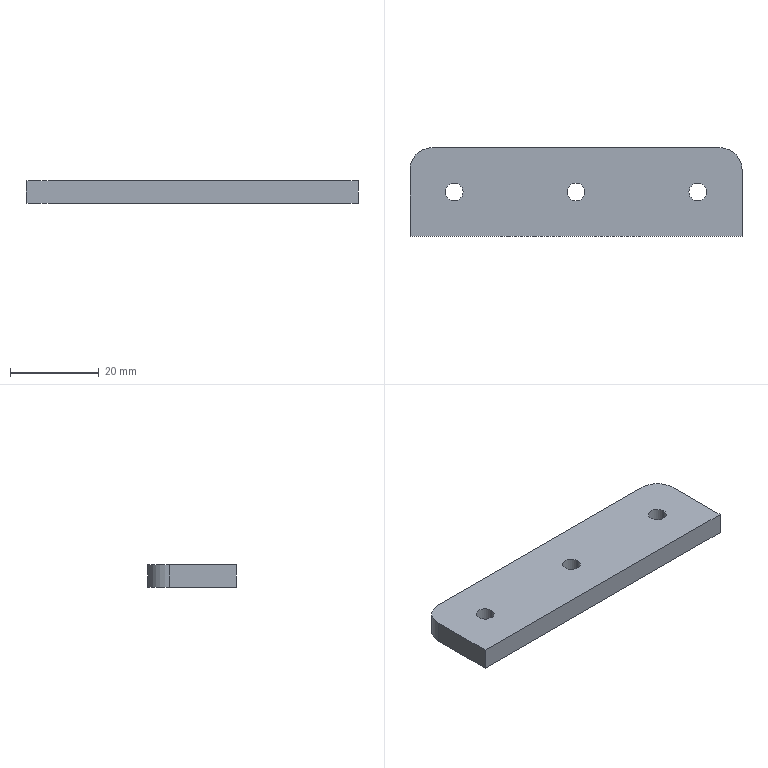Part | SolidWorks | features Extrusion 1, Fillet 1 | 1 solid | 14 faces | box 75 x 20 x 5 mm | volume 7258 mm3 | cylinder 8 | plane 6 | commonest cylinder face diameters 4 x6 10 x2
STEP:
#1=CARTESIAN_POINT('',(63.,-10.,5.));
#2=VERTEX_POINT('',#1);
#3=CARTESIAN_POINT('',(67.,-10.,5.));
#4=VERTEX_POINT('',#3);
#5=CARTESIAN_POINT('',(65.,-10.,5.));
#6=DIRECTION('',(0.,0.,1.));
#7=DIRECTION('',(1.,0.,0.));
#8=AXIS2_PLACEMENT_3D('',#5,#6,#7);
#9=CIRCLE('',#8,2.);
#10=EDGE_CURVE('',#2,#4,#9,.T.);
#11=ORIENTED_EDGE('',*,*,#10,.T.);
#12=CARTESIAN_POINT('',(67.,-10.,0.));
#13=VERTEX_POINT('',#12);
#14=CARTESIAN_POINT('',(67.,-10.,5.));
#15=DIRECTION('',(0.,0.,-1.));
#16=VECTOR('',#15,1000.);
#17=LINE('',#14,#16);
#18=EDGE_CURVE('',#4,#13,#17,.T.);
#19=ORIENTED_EDGE('',*,*,#18,.T.);
#20=CARTESIAN_POINT('',(63.,-10.,0.));
#21=VERTEX_POINT('',#20);
#22=CARTESIAN_POINT('',(65.,-10.,0.));
#23=DIRECTION('',(0.,0.,1.));
#24=DIRECTION('',(1.,0.,0.));
#25=AXIS2_PLACEMENT_3D('',#22,#23,#24);
#26=CIRCLE('',#25,2.);
#27=EDGE_CURVE('',#21,#13,#26,.T.);
#28=ORIENTED_EDGE('',*,*,#27,.F.);
#29=CARTESIAN_POINT('',(63.,-10.,5.));
#30=DIRECTION('',(0.,0.,-1.));
#31=VECTOR('',#30,1000.);
#32=LINE('',#29,#31);
#33=EDGE_CURVE('',#2,#21,#32,.T.);
#34=ORIENTED_EDGE('',*,*,#33,.F.);
#35=EDGE_LOOP('',(#11,#19,#28,#34));
#36=FACE_OUTER_BOUND('',#35,.T.);
#37=CARTESIAN_POINT('',(65.,-10.,5.));
#38=DIRECTION('',(0.,0.,-1.));
#39=DIRECTION('',(-1.,0.,0.));
#40=AXIS2_PLACEMENT_3D('',#37,#38,#39);
#41=CYLINDRICAL_SURFACE('',#40,2.);
#42=ADVANCED_FACE('',(#36),#41,.F.);
#43=CARTESIAN_POINT('',(35.5,-10.,5.));
#44=VERTEX_POINT('',#43);
#45=CARTESIAN_POINT('',(39.5,-10.,5.));
#46=VERTEX_POINT('',#45);
#47=CARTESIAN_POINT('',(37.5,-10.,5.));
#48=DIRECTION('',(0.,0.,1.));
#49=DIRECTION('',(1.,0.,0.));
#50=AXIS2_PLACEMENT_3D('',#47,#48,#49);
#51=CIRCLE('',#50,2.);
#52=EDGE_CURVE('',#44,#46,#51,.T.);
#53=ORIENTED_EDGE('',*,*,#52,.T.);
#54=CARTESIAN_POINT('',(39.5,-10.,0.));
#55=VERTEX_POINT('',#54);
#56=CARTESIAN_POINT('',(39.5,-10.,5.));
#57=DIRECTION('',(0.,0.,-1.));
#58=VECTOR('',#57,1000.);
#59=LINE('',#56,#58);
#60=EDGE_CURVE('',#46,#55,#59,.T.);
#61=ORIENTED_EDGE('',*,*,#60,.T.);
#62=CARTESIAN_POINT('',(35.5,-10.,0.));
#63=VERTEX_POINT('',#62);
#64=CARTESIAN_POINT('',(37.5,-10.,0.));
#65=DIRECTION('',(0.,0.,1.));
#66=DIRECTION('',(1.,0.,0.));
#67=AXIS2_PLACEMENT_3D('',#64,#65,#66);
#68=CIRCLE('',#67,2.);
#69=EDGE_CURVE('',#63,#55,#68,.T.);
#70=ORIENTED_EDGE('',*,*,#69,.F.);
#71=CARTESIAN_POINT('',(35.5,-10.,5.));
#72=DIRECTION('',(0.,0.,-1.));
#73=VECTOR('',#72,1000.);
#74=LINE('',#71,#73);
#75=EDGE_CURVE('',#44,#63,#74,.T.);
#76=ORIENTED_EDGE('',*,*,#75,.F.);
#77=EDGE_LOOP('',(#53,#61,#70,#76));
#78=FACE_OUTER_BOUND('',#77,.T.);
#79=CARTESIAN_POINT('',(37.5,-10.,5.));
#80=DIRECTION('',(0.,0.,-1.));
#81=DIRECTION('',(-1.,0.,0.));
#82=AXIS2_PLACEMENT_3D('',#79,#80,#81);
#83=CYLINDRICAL_SURFACE('',#82,2.);
#84=ADVANCED_FACE('',(#78),#83,.F.);
#85=CARTESIAN_POINT('',(8.,-10.,5.));
#86=VERTEX_POINT('',#85);
#87=CARTESIAN_POINT('',(12.,-10.,5.));
#88=VERTEX_POINT('',#87);
#89=CARTESIAN_POINT('',(10.,-10.,5.));
#90=DIRECTION('',(0.,0.,1.));
#91=DIRECTION('',(1.,0.,0.));
#92=AXIS2_PLACEMENT_3D('',#89,#90,#91);
#93=CIRCLE('',#92,2.);
#94=EDGE_CURVE('',#86,#88,#93,.T.);
#95=ORIENTED_EDGE('',*,*,#94,.T.);
#96=CARTESIAN_POINT('',(12.,-10.,0.));
#97=VERTEX_POINT('',#96);
#98=CARTESIAN_POINT('',(12.,-10.,5.));
#99=DIRECTION('',(0.,0.,-1.));
#100=VECTOR('',#99,1000.);
#101=LINE('',#98,#100);
#102=EDGE_CURVE('',#88,#97,#101,.T.);
#103=ORIENTED_EDGE('',*,*,#102,.T.);
#104=CARTESIAN_POINT('',(8.,-10.,0.));
#105=VERTEX_POINT('',#104);
#106=CARTESIAN_POINT('',(10.,-10.,0.));
#107=DIRECTION('',(0.,0.,1.));
#108=DIRECTION('',(1.,0.,0.));
#109=AXIS2_PLACEMENT_3D('',#106,#107,#108);
#110=CIRCLE('',#109,2.);
#111=EDGE_CURVE('',#105,#97,#110,.T.);
#112=ORIENTED_EDGE('',*,*,#111,.F.);
#113=CARTESIAN_POINT('',(8.,-10.,5.));
#114=DIRECTION('',(0.,0.,-1.));
#115=VECTOR('',#114,1000.);
#116=LINE('',#113,#115);
#117=EDGE_CURVE('',#86,#105,#116,.T.);
#118=ORIENTED_EDGE('',*,*,#117,.F.);
#119=EDGE_LOOP('',(#95,#103,#112,#118));
#120=FACE_OUTER_BOUND('',#119,.T.);
#121=CARTESIAN_POINT('',(10.,-10.,5.));
#122=DIRECTION('',(0.,0.,-1.));
#123=DIRECTION('',(-1.,0.,0.));
#124=AXIS2_PLACEMENT_3D('',#121,#122,#123);
#125=CYLINDRICAL_SURFACE('',#124,2.);
#126=ADVANCED_FACE('',(#120),#125,.F.);
#127=ORIENTED_EDGE('',*,*,#52,.F.);
#128=CARTESIAN_POINT('',(37.5,-10.,5.));
#129=DIRECTION('',(0.,0.,1.));
#130=DIRECTION('',(1.,0.,0.));
#131=AXIS2_PLACEMENT_3D('',#128,#129,#130);
#132=CIRCLE('',#131,2.);
#133=EDGE_CURVE('',#46,#44,#132,.T.);
#134=ORIENTED_EDGE('',*,*,#133,.F.);
#135=EDGE_LOOP('',(#127,#134));
#136=FACE_BOUND('',#135,.T.);
#137=CARTESIAN_POINT('',(75.,-20.,5.));
#138=VERTEX_POINT('',#137);
#139=CARTESIAN_POINT('',(75.,-5.,5.));
#140=VERTEX_POINT('',#139);
#141=CARTESIAN_POINT('',(75.,0.,5.));
#142=DIRECTION('',(0.,1.,0.));
#143=VECTOR('',#142,1000.);
#144=LINE('',#141,#143);
#145=EDGE_CURVE('',#138,#140,#144,.T.);
#146=ORIENTED_EDGE('',*,*,#145,.T.);
#147=CARTESIAN_POINT('',(70.,0.,5.));
#148=VERTEX_POINT('',#147);
#149=CARTESIAN_POINT('',(70.,-5.,5.));
#150=DIRECTION('',(0.,0.,1.));
#151=DIRECTION('',(1.,0.,0.));
#152=AXIS2_PLACEMENT_3D('',#149,#150,#151);
#153=CIRCLE('',#152,5.);
#154=EDGE_CURVE('',#140,#148,#153,.T.);
#155=ORIENTED_EDGE('',*,*,#154,.T.);
#156=CARTESIAN_POINT('',(5.,0.,5.));
#157=VERTEX_POINT('',#156);
#158=CARTESIAN_POINT('',(0.,0.,5.));
#159=DIRECTION('',(-1.,0.,0.));
#160=VECTOR('',#159,1000.);
#161=LINE('',#158,#160);
#162=EDGE_CURVE('',#148,#157,#161,.T.);
#163=ORIENTED_EDGE('',*,*,#162,.T.);
#164=CARTESIAN_POINT('',(0.,-5.,5.));
#165=VERTEX_POINT('',#164);
#166=CARTESIAN_POINT('',(5.,-5.,5.));
#167=DIRECTION('',(0.,0.,1.));
#168=DIRECTION('',(1.,0.,0.));
#169=AXIS2_PLACEMENT_3D('',#166,#167,#168);
#170=CIRCLE('',#169,5.);
#171=EDGE_CURVE('',#157,#165,#170,.T.);
#172=ORIENTED_EDGE('',*,*,#171,.T.);
#173=CARTESIAN_POINT('',(0.,-20.,5.));
#174=VERTEX_POINT('',#173);
#175=CARTESIAN_POINT('',(0.,0.,5.));
#176=DIRECTION('',(0.,-1.,0.));
#177=VECTOR('',#176,1000.);
#178=LINE('',#175,#177);
#179=EDGE_CURVE('',#165,#174,#178,.T.);
#180=ORIENTED_EDGE('',*,*,#179,.T.);
#181=CARTESIAN_POINT('',(0.,-20.,5.));
#182=DIRECTION('',(1.,0.,0.));
#183=VECTOR('',#182,1000.);
#184=LINE('',#181,#183);
#185=EDGE_CURVE('',#174,#138,#184,.T.);
#186=ORIENTED_EDGE('',*,*,#185,.T.);
#187=EDGE_LOOP('',(#146,#155,#163,#172,#180,#186));
#188=FACE_OUTER_BOUND('',#187,.T.);
#189=ORIENTED_EDGE('',*,*,#94,.F.);
#190=CARTESIAN_POINT('',(10.,-10.,5.));
#191=DIRECTION('',(0.,0.,1.));
#192=DIRECTION('',(1.,0.,0.));
#193=AXIS2_PLACEMENT_3D('',#190,#191,#192);
#194=CIRCLE('',#193,2.);
#195=EDGE_CURVE('',#88,#86,#194,.T.);
#196=ORIENTED_EDGE('',*,*,#195,.F.);
#197=EDGE_LOOP('',(#189,#196));
#198=FACE_BOUND('',#197,.T.);
#199=ORIENTED_EDGE('',*,*,#10,.F.);
#200=CARTESIAN_POINT('',(65.,-10.,5.));
#201=DIRECTION('',(0.,0.,1.));
#202=DIRECTION('',(1.,0.,0.));
#203=AXIS2_PLACEMENT_3D('',#200,#201,#202);
#204=CIRCLE('',#203,2.);
#205=EDGE_CURVE('',#4,#2,#204,.T.);
#206=ORIENTED_EDGE('',*,*,#205,.F.);
#207=EDGE_LOOP('',(#199,#206));
#208=FACE_BOUND('',#207,.T.);
#209=CARTESIAN_POINT('',(0.,0.,5.));
#210=DIRECTION('',(0.,0.,1.));
#211=DIRECTION('',(1.,0.,0.));
#212=AXIS2_PLACEMENT_3D('',#209,#210,#211);
#213=PLANE('',#212);
#214=ADVANCED_FACE('',(#136,#188,#198,#208),#213,.T.);
#215=CARTESIAN_POINT('',(70.,0.,0.));
#216=VERTEX_POINT('',#215);
#217=CARTESIAN_POINT('',(5.,0.,0.));
#218=VERTEX_POINT('',#217);
#219=CARTESIAN_POINT('',(0.,0.,0.));
#220=DIRECTION('',(-1.,0.,0.));
#221=VECTOR('',#220,1000.);
#222=LINE('',#219,#221);
#223=EDGE_CURVE('',#216,#218,#222,.T.);
#224=ORIENTED_EDGE('',*,*,#223,.F.);
#225=CARTESIAN_POINT('',(75.,-5.,0.));
#226=VERTEX_POINT('',#225);
#227=CARTESIAN_POINT('',(70.,-5.,0.));
#228=DIRECTION('',(0.,0.,-1.));
#229=DIRECTION('',(1.,0.,0.));
#230=AXIS2_PLACEMENT_3D('',#227,#228,#229);
#231=CIRCLE('',#230,5.);
#232=EDGE_CURVE('',#216,#226,#231,.T.);
#233=ORIENTED_EDGE('',*,*,#232,.T.);
#234=CARTESIAN_POINT('',(75.,-20.,0.));
#235=VERTEX_POINT('',#234);
#236=CARTESIAN_POINT('',(75.,0.,0.));
#237=DIRECTION('',(0.,1.,0.));
#238=VECTOR('',#237,1000.);
#239=LINE('',#236,#238);
#240=EDGE_CURVE('',#235,#226,#239,.T.);
#241=ORIENTED_EDGE('',*,*,#240,.F.);
#242=CARTESIAN_POINT('',(0.,-20.,0.));
#243=VERTEX_POINT('',#242);
#244=CARTESIAN_POINT('',(0.,-20.,0.));
#245=DIRECTION('',(1.,0.,0.));
#246=VECTOR('',#245,1000.);
#247=LINE('',#244,#246);
#248=EDGE_CURVE('',#243,#235,#247,.T.);
#249=ORIENTED_EDGE('',*,*,#248,.F.);
#250=CARTESIAN_POINT('',(0.,-5.,0.));
#251=VERTEX_POINT('',#250);
#252=CARTESIAN_POINT('',(0.,0.,0.));
#253=DIRECTION('',(0.,-1.,0.));
#254=VECTOR('',#253,1000.);
#255=LINE('',#252,#254);
#256=EDGE_CURVE('',#251,#243,#255,.T.);
#257=ORIENTED_EDGE('',*,*,#256,.F.);
#258=CARTESIAN_POINT('',(5.,-5.,0.));
#259=DIRECTION('',(0.,0.,-1.));
#260=DIRECTION('',(1.,0.,0.));
#261=AXIS2_PLACEMENT_3D('',#258,#259,#260);
#262=CIRCLE('',#261,5.);
#263=EDGE_CURVE('',#251,#218,#262,.T.);
#264=ORIENTED_EDGE('',*,*,#263,.T.);
#265=EDGE_LOOP('',(#224,#233,#241,#249,#257,#264));
#266=FACE_OUTER_BOUND('',#265,.T.);
#267=ORIENTED_EDGE('',*,*,#111,.T.);
#268=CARTESIAN_POINT('',(10.,-10.,0.));
#269=DIRECTION('',(0.,0.,1.));
#270=DIRECTION('',(1.,0.,0.));
#271=AXIS2_PLACEMENT_3D('',#268,#269,#270);
#272=CIRCLE('',#271,2.);
#273=EDGE_CURVE('',#97,#105,#272,.T.);
#274=ORIENTED_EDGE('',*,*,#273,.T.);
#275=EDGE_LOOP('',(#267,#274));
#276=FACE_BOUND('',#275,.T.);
#277=ORIENTED_EDGE('',*,*,#69,.T.);
#278=CARTESIAN_POINT('',(37.5,-10.,0.));
#279=DIRECTION('',(0.,0.,1.));
#280=DIRECTION('',(1.,0.,0.));
#281=AXIS2_PLACEMENT_3D('',#278,#279,#280);
#282=CIRCLE('',#281,2.);
#283=EDGE_CURVE('',#55,#63,#282,.T.);
#284=ORIENTED_EDGE('',*,*,#283,.T.);
#285=EDGE_LOOP('',(#277,#284));
#286=FACE_BOUND('',#285,.T.);
#287=ORIENTED_EDGE('',*,*,#27,.T.);
#288=CARTESIAN_POINT('',(65.,-10.,0.));
#289=DIRECTION('',(0.,0.,1.));
#290=DIRECTION('',(1.,0.,0.));
#291=AXIS2_PLACEMENT_3D('',#288,#289,#290);
#292=CIRCLE('',#291,2.);
#293=EDGE_CURVE('',#13,#21,#292,.T.);
#294=ORIENTED_EDGE('',*,*,#293,.T.);
#295=EDGE_LOOP('',(#287,#294));
#296=FACE_BOUND('',#295,.T.);
#297=CARTESIAN_POINT('',(0.,0.,0.));
#298=DIRECTION('',(0.,0.,1.));
#299=DIRECTION('',(1.,0.,0.));
#300=AXIS2_PLACEMENT_3D('',#297,#298,#299);
#301=PLANE('',#300);
#302=ADVANCED_FACE('',(#266,#276,#286,#296),#301,.F.);
#303=ORIENTED_EDGE('',*,*,#179,.F.);
#304=CARTESIAN_POINT('',(0.,-5.,5.));
#305=DIRECTION('',(0.,0.,-1.));
#306=VECTOR('',#305,1000.);
#307=LINE('',#304,#306);
#308=EDGE_CURVE('',#165,#251,#307,.T.);
#309=ORIENTED_EDGE('',*,*,#308,.T.);
#310=ORIENTED_EDGE('',*,*,#256,.T.);
#311=CARTESIAN_POINT('',(0.,-20.,5.));
#312=DIRECTION('',(0.,0.,-1.));
#313=VECTOR('',#312,1000.);
#314=LINE('',#311,#313);
#315=EDGE_CURVE('',#174,#243,#314,.T.);
#316=ORIENTED_EDGE('',*,*,#315,.F.);
#317=EDGE_LOOP('',(#303,#309,#310,#316));
#318=FACE_OUTER_BOUND('',#317,.T.);
#319=CARTESIAN_POINT('',(0.,0.,5.));
#320=DIRECTION('',(1.,0.,0.));
#321=DIRECTION('',(0.,1.,0.));
#322=AXIS2_PLACEMENT_3D('',#319,#320,#321);
#323=PLANE('',#322);
#324=ADVANCED_FACE('',(#318),#323,.F.);
#325=ORIENTED_EDGE('',*,*,#248,.T.);
#326=CARTESIAN_POINT('',(75.,-20.,5.));
#327=DIRECTION('',(0.,0.,-1.));
#328=VECTOR('',#327,1000.);
#329=LINE('',#326,#328);
#330=EDGE_CURVE('',#138,#235,#329,.T.);
#331=ORIENTED_EDGE('',*,*,#330,.F.);
#332=ORIENTED_EDGE('',*,*,#185,.F.);
#333=ORIENTED_EDGE('',*,*,#315,.T.);
#334=EDGE_LOOP('',(#325,#331,#332,#333));
#335=FACE_OUTER_BOUND('',#334,.T.);
#336=CARTESIAN_POINT('',(0.,-20.,5.));
#337=DIRECTION('',(0.,1.,0.));
#338=DIRECTION('',(0.,0.,1.));
#339=AXIS2_PLACEMENT_3D('',#336,#337,#338);
#340=PLANE('',#339);
#341=ADVANCED_FACE('',(#335),#340,.F.);
#342=ORIENTED_EDGE('',*,*,#240,.T.);
#343=CARTESIAN_POINT('',(75.,-5.,5.));
#344=DIRECTION('',(0.,0.,1.));
#345=VECTOR('',#344,1000.);
#346=LINE('',#343,#345);
#347=EDGE_CURVE('',#226,#140,#346,.T.);
#348=ORIENTED_EDGE('',*,*,#347,.T.);
#349=ORIENTED_EDGE('',*,*,#145,.F.);
#350=ORIENTED_EDGE('',*,*,#330,.T.);
#351=EDGE_LOOP('',(#342,#348,#349,#350));
#352=FACE_OUTER_BOUND('',#351,.T.);
#353=CARTESIAN_POINT('',(75.,0.,5.));
#354=DIRECTION('',(-1.,0.,0.));
#355=DIRECTION('',(0.,0.,1.));
#356=AXIS2_PLACEMENT_3D('',#353,#354,#355);
#357=PLANE('',#356);
#358=ADVANCED_FACE('',(#352),#357,.F.);
#359=ORIENTED_EDGE('',*,*,#162,.F.);
#360=CARTESIAN_POINT('',(70.,0.,5.));
#361=DIRECTION('',(0.,0.,-1.));
#362=VECTOR('',#361,1000.);
#363=LINE('',#360,#362);
#364=EDGE_CURVE('',#148,#216,#363,.T.);
#365=ORIENTED_EDGE('',*,*,#364,.T.);
#366=ORIENTED_EDGE('',*,*,#223,.T.);
#367=CARTESIAN_POINT('',(5.,0.,5.));
#368=DIRECTION('',(0.,0.,1.));
#369=VECTOR('',#368,1000.);
#370=LINE('',#367,#369);
#371=EDGE_CURVE('',#218,#157,#370,.T.);
#372=ORIENTED_EDGE('',*,*,#371,.T.);
#373=EDGE_LOOP('',(#359,#365,#366,#372));
#374=FACE_OUTER_BOUND('',#373,.T.);
#375=CARTESIAN_POINT('',(0.,0.,5.));
#376=DIRECTION('',(0.,-1.,0.));
#377=DIRECTION('',(0.,0.,-1.));
#378=AXIS2_PLACEMENT_3D('',#375,#376,#377);
#379=PLANE('',#378);
#380=ADVANCED_FACE('',(#374),#379,.F.);
#381=ORIENTED_EDGE('',*,*,#102,.F.);
#382=ORIENTED_EDGE('',*,*,#195,.T.);
#383=ORIENTED_EDGE('',*,*,#117,.T.);
#384=ORIENTED_EDGE('',*,*,#273,.F.);
#385=EDGE_LOOP('',(#381,#382,#383,#384));
#386=FACE_OUTER_BOUND('',#385,.T.);
#387=CARTESIAN_POINT('',(10.,-10.,5.));
#388=DIRECTION('',(0.,0.,-1.));
#389=DIRECTION('',(-1.,0.,0.));
#390=AXIS2_PLACEMENT_3D('',#387,#388,#389);
#391=CYLINDRICAL_SURFACE('',#390,2.);
#392=ADVANCED_FACE('',(#386),#391,.F.);
#393=ORIENTED_EDGE('',*,*,#60,.F.);
#394=ORIENTED_EDGE('',*,*,#133,.T.);
#395=ORIENTED_EDGE('',*,*,#75,.T.);
#396=ORIENTED_EDGE('',*,*,#283,.F.);
#397=EDGE_LOOP('',(#393,#394,#395,#396));
#398=FACE_OUTER_BOUND('',#397,.T.);
#399=CARTESIAN_POINT('',(37.5,-10.,5.));
#400=DIRECTION('',(0.,0.,-1.));
#401=DIRECTION('',(-1.,0.,0.));
#402=AXIS2_PLACEMENT_3D('',#399,#400,#401);
#403=CYLINDRICAL_SURFACE('',#402,2.);
#404=ADVANCED_FACE('',(#398),#403,.F.);
#405=ORIENTED_EDGE('',*,*,#18,.F.);
#406=ORIENTED_EDGE('',*,*,#205,.T.);
#407=ORIENTED_EDGE('',*,*,#33,.T.);
#408=ORIENTED_EDGE('',*,*,#293,.F.);
#409=EDGE_LOOP('',(#405,#406,#407,#408));
#410=FACE_OUTER_BOUND('',#409,.T.);
#411=CARTESIAN_POINT('',(65.,-10.,5.));
#412=DIRECTION('',(0.,0.,-1.));
#413=DIRECTION('',(-1.,0.,0.));
#414=AXIS2_PLACEMENT_3D('',#411,#412,#413);
#415=CYLINDRICAL_SURFACE('',#414,2.);
#416=ADVANCED_FACE('',(#410),#415,.F.);
#417=ORIENTED_EDGE('',*,*,#154,.F.);
#418=ORIENTED_EDGE('',*,*,#347,.F.);
#419=ORIENTED_EDGE('',*,*,#232,.F.);
#420=ORIENTED_EDGE('',*,*,#364,.F.);
#421=EDGE_LOOP('',(#417,#418,#419,#420));
#422=FACE_OUTER_BOUND('',#421,.T.);
#423=CARTESIAN_POINT('',(70.,-5.,5.));
#424=DIRECTION('',(0.,0.,-1.));
#425=DIRECTION('',(-1.,0.,0.));
#426=AXIS2_PLACEMENT_3D('',#423,#424,#425);
#427=CYLINDRICAL_SURFACE('',#426,5.);
#428=ADVANCED_FACE('',(#422),#427,.T.);
#429=ORIENTED_EDGE('',*,*,#171,.F.);
#430=ORIENTED_EDGE('',*,*,#371,.F.);
#431=ORIENTED_EDGE('',*,*,#263,.F.);
#432=ORIENTED_EDGE('',*,*,#308,.F.);
#433=EDGE_LOOP('',(#429,#430,#431,#432));
#434=FACE_OUTER_BOUND('',#433,.T.);
#435=CARTESIAN_POINT('',(5.,-5.,5.));
#436=DIRECTION('',(0.,0.,-1.));
#437=DIRECTION('',(-1.,0.,0.));
#438=AXIS2_PLACEMENT_3D('',#435,#436,#437);
#439=CYLINDRICAL_SURFACE('',#438,5.);
#440=ADVANCED_FACE('',(#434),#439,.T.);
#441=CLOSED_SHELL('',(#42,#84,#126,#214,#302,#324,#341,#358,#380,#392,#404,#416,#428,#440));
#442=MANIFOLD_SOLID_BREP('',#441);
#443=CARTESIAN_POINT('',(0.,0.,0.));
#444=DIRECTION('',(0.,0.,1.));
#445=DIRECTION('',(1.,0.,0.));
#446=AXIS2_PLACEMENT_3D('',#443,#444,#445);
#447=(LENGTH_UNIT()NAMED_UNIT(*)SI_UNIT(.MILLI.,.METRE.));
#448=UNCERTAINTY_MEASURE_WITH_UNIT(LENGTH_MEASURE(0.00001),#447,'','');
#449=(NAMED_UNIT(*)PLANE_ANGLE_UNIT()SI_UNIT($,.RADIAN.));
#450=(NAMED_UNIT(*)SI_UNIT($,.STERADIAN.)SOLID_ANGLE_UNIT());
#451=(GEOMETRIC_REPRESENTATION_CONTEXT(3)GLOBAL_UNCERTAINTY_ASSIGNED_CONTEXT((#448))GLOBAL_UNIT_ASSIGNED_CONTEXT((#447,#449,#450))REPRESENTATION_CONTEXT('',''));
#452=ADVANCED_BREP_SHAPE_REPRESENTATION('',(#442,#446),#451);